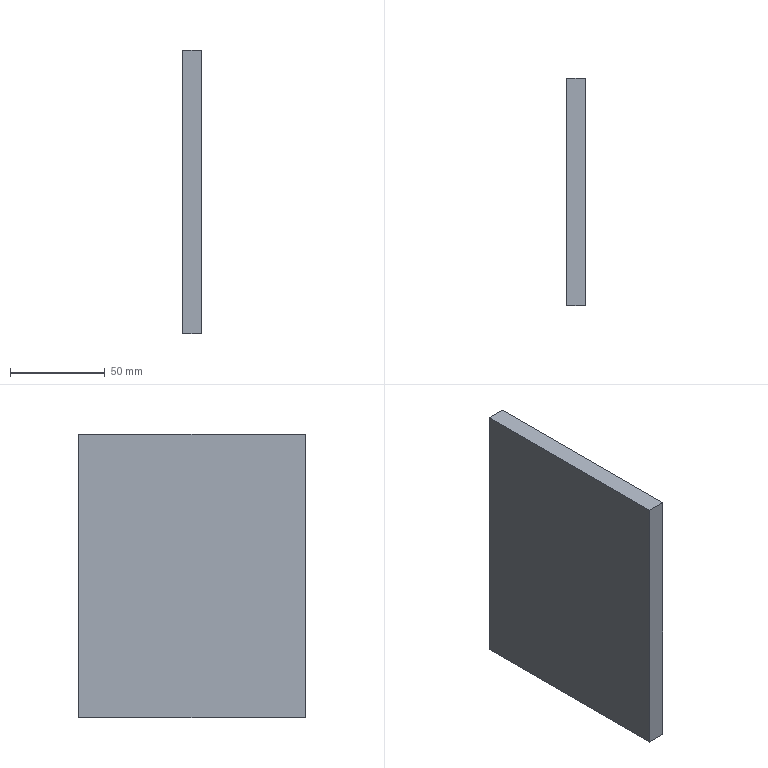Part | NX | 1 solid | 6 faces | box 10 x 120 x 150 mm | volume 180000 mm3 | plane 6
STEP:
#1=CARTESIAN_POINT('',(0.,-120.,0.));
#2=VERTEX_POINT('',#1);
#3=CARTESIAN_POINT('',(0.,-120.,-150.));
#4=VERTEX_POINT('',#3);
#5=CARTESIAN_POINT('',(0.,-120.,0.));
#6=DIRECTION('',(0.,0.,-1.));
#7=VECTOR('',#6,1.);
#8=LINE('',#5,#7);
#9=EDGE_CURVE('',#2,#4,#8,.T.);
#10=ORIENTED_EDGE('',*,*,#9,.T.);
#11=CARTESIAN_POINT('',(10.,-120.,-150.));
#12=VERTEX_POINT('',#11);
#13=CARTESIAN_POINT('',(10.,-120.,-150.));
#14=DIRECTION('',(-1.,0.,0.));
#15=VECTOR('',#14,1.);
#16=LINE('',#13,#15);
#17=EDGE_CURVE('',#12,#4,#16,.T.);
#18=ORIENTED_EDGE('',*,*,#17,.F.);
#19=CARTESIAN_POINT('',(10.,-120.,0.));
#20=VERTEX_POINT('',#19);
#21=CARTESIAN_POINT('',(10.,-120.,0.));
#22=DIRECTION('',(0.,0.,-1.));
#23=VECTOR('',#22,1.);
#24=LINE('',#21,#23);
#25=EDGE_CURVE('',#20,#12,#24,.T.);
#26=ORIENTED_EDGE('',*,*,#25,.F.);
#27=CARTESIAN_POINT('',(10.,-120.,0.));
#28=DIRECTION('',(-1.,0.,0.));
#29=VECTOR('',#28,1.);
#30=LINE('',#27,#29);
#31=EDGE_CURVE('',#20,#2,#30,.T.);
#32=ORIENTED_EDGE('',*,*,#31,.T.);
#33=EDGE_LOOP('',(#10,#18,#26,#32));
#34=FACE_OUTER_BOUND('',#33,.T.);
#35=CARTESIAN_POINT('',(10.,-120.,0.));
#36=DIRECTION('',(0.,1.,0.));
#37=DIRECTION('',(0.,0.,-1.));
#38=AXIS2_PLACEMENT_3D('',#35,#36,#37);
#39=PLANE('',#38);
#40=ADVANCED_FACE('',(#34),#39,.F.);
#41=CARTESIAN_POINT('',(0.,0.,-150.));
#42=VERTEX_POINT('',#41);
#43=CARTESIAN_POINT('',(0.,-120.,-150.));
#44=DIRECTION('',(0.,1.,0.));
#45=VECTOR('',#44,1.);
#46=LINE('',#43,#45);
#47=EDGE_CURVE('',#4,#42,#46,.T.);
#48=ORIENTED_EDGE('',*,*,#47,.T.);
#49=CARTESIAN_POINT('',(10.,0.,-150.));
#50=VERTEX_POINT('',#49);
#51=CARTESIAN_POINT('',(10.,0.,-150.));
#52=DIRECTION('',(-1.,0.,0.));
#53=VECTOR('',#52,1.);
#54=LINE('',#51,#53);
#55=EDGE_CURVE('',#50,#42,#54,.T.);
#56=ORIENTED_EDGE('',*,*,#55,.F.);
#57=CARTESIAN_POINT('',(10.,-120.,-150.));
#58=DIRECTION('',(0.,1.,0.));
#59=VECTOR('',#58,1.);
#60=LINE('',#57,#59);
#61=EDGE_CURVE('',#12,#50,#60,.T.);
#62=ORIENTED_EDGE('',*,*,#61,.F.);
#63=ORIENTED_EDGE('',*,*,#17,.T.);
#64=EDGE_LOOP('',(#48,#56,#62,#63));
#65=FACE_OUTER_BOUND('',#64,.T.);
#66=CARTESIAN_POINT('',(10.,-120.,-150.));
#67=DIRECTION('',(0.,0.,1.));
#68=DIRECTION('',(0.,1.,0.));
#69=AXIS2_PLACEMENT_3D('',#66,#67,#68);
#70=PLANE('',#69);
#71=ADVANCED_FACE('',(#65),#70,.F.);
#72=CARTESIAN_POINT('',(0.,0.,0.));
#73=VERTEX_POINT('',#72);
#74=CARTESIAN_POINT('',(0.,0.,-150.));
#75=DIRECTION('',(0.,0.,1.));
#76=VECTOR('',#75,1.);
#77=LINE('',#74,#76);
#78=EDGE_CURVE('',#42,#73,#77,.T.);
#79=ORIENTED_EDGE('',*,*,#78,.T.);
#80=CARTESIAN_POINT('',(10.,0.,0.));
#81=VERTEX_POINT('',#80);
#82=CARTESIAN_POINT('',(10.,0.,0.));
#83=DIRECTION('',(-1.,0.,0.));
#84=VECTOR('',#83,1.);
#85=LINE('',#82,#84);
#86=EDGE_CURVE('',#81,#73,#85,.T.);
#87=ORIENTED_EDGE('',*,*,#86,.F.);
#88=CARTESIAN_POINT('',(10.,0.,-150.));
#89=DIRECTION('',(0.,0.,1.));
#90=VECTOR('',#89,1.);
#91=LINE('',#88,#90);
#92=EDGE_CURVE('',#50,#81,#91,.T.);
#93=ORIENTED_EDGE('',*,*,#92,.F.);
#94=ORIENTED_EDGE('',*,*,#55,.T.);
#95=EDGE_LOOP('',(#79,#87,#93,#94));
#96=FACE_OUTER_BOUND('',#95,.T.);
#97=CARTESIAN_POINT('',(10.,0.,-150.));
#98=DIRECTION('',(0.,-1.,0.));
#99=DIRECTION('',(0.,0.,1.));
#100=AXIS2_PLACEMENT_3D('',#97,#98,#99);
#101=PLANE('',#100);
#102=ADVANCED_FACE('',(#96),#101,.F.);
#103=CARTESIAN_POINT('',(0.,0.,0.));
#104=DIRECTION('',(0.,-1.,0.));
#105=VECTOR('',#104,1.);
#106=LINE('',#103,#105);
#107=EDGE_CURVE('',#73,#2,#106,.T.);
#108=ORIENTED_EDGE('',*,*,#107,.T.);
#109=ORIENTED_EDGE('',*,*,#31,.F.);
#110=CARTESIAN_POINT('',(10.,0.,0.));
#111=DIRECTION('',(0.,-1.,0.));
#112=VECTOR('',#111,1.);
#113=LINE('',#110,#112);
#114=EDGE_CURVE('',#81,#20,#113,.T.);
#115=ORIENTED_EDGE('',*,*,#114,.F.);
#116=ORIENTED_EDGE('',*,*,#86,.T.);
#117=EDGE_LOOP('',(#108,#109,#115,#116));
#118=FACE_OUTER_BOUND('',#117,.T.);
#119=CARTESIAN_POINT('',(10.,0.,0.));
#120=DIRECTION('',(0.,0.,-1.));
#121=DIRECTION('',(0.,-1.,0.));
#122=AXIS2_PLACEMENT_3D('',#119,#120,#121);
#123=PLANE('',#122);
#124=ADVANCED_FACE('',(#118),#123,.F.);
#125=ORIENTED_EDGE('',*,*,#25,.T.);
#126=ORIENTED_EDGE('',*,*,#61,.T.);
#127=ORIENTED_EDGE('',*,*,#92,.T.);
#128=ORIENTED_EDGE('',*,*,#114,.T.);
#129=EDGE_LOOP('',(#125,#126,#127,#128));
#130=FACE_OUTER_BOUND('',#129,.T.);
#131=CARTESIAN_POINT('',(10.,0.,0.));
#132=DIRECTION('',(1.,0.,0.));
#133=DIRECTION('',(0.,0.,1.));
#134=AXIS2_PLACEMENT_3D('',#131,#132,#133);
#135=PLANE('',#134);
#136=ADVANCED_FACE('',(#130),#135,.T.);
#137=ORIENTED_EDGE('',*,*,#9,.F.);
#138=ORIENTED_EDGE('',*,*,#107,.F.);
#139=ORIENTED_EDGE('',*,*,#78,.F.);
#140=ORIENTED_EDGE('',*,*,#47,.F.);
#141=EDGE_LOOP('',(#137,#138,#139,#140));
#142=FACE_OUTER_BOUND('',#141,.T.);
#143=CARTESIAN_POINT('',(0.,0.,0.));
#144=DIRECTION('',(1.,0.,0.));
#145=DIRECTION('',(0.,0.,1.));
#146=AXIS2_PLACEMENT_3D('',#143,#144,#145);
#147=PLANE('',#146);
#148=ADVANCED_FACE('',(#142),#147,.F.);
#149=CLOSED_SHELL('',(#40,#71,#102,#124,#136,#148));
#150=MANIFOLD_SOLID_BREP('',#149);
#151=(LENGTH_UNIT()NAMED_UNIT(*)SI_UNIT(.MILLI.,.METRE.));
#152=UNCERTAINTY_MEASURE_WITH_UNIT(LENGTH_MEASURE(0.00002),#151,'','');
#153=(NAMED_UNIT(*)PLANE_ANGLE_UNIT()SI_UNIT($,.RADIAN.));
#154=PLANE_ANGLE_MEASURE_WITH_UNIT(PLANE_ANGLE_MEASURE(0.01745),#153);
#155=DIMENSIONAL_EXPONENTS(0.,0.,0.,0.,0.,0.,0.);
#156=(CONVERSION_BASED_UNIT('DEGREE',#154)NAMED_UNIT(#155)PLANE_ANGLE_UNIT());
#157=(NAMED_UNIT(*)SI_UNIT($,.STERADIAN.)SOLID_ANGLE_UNIT());
#158=(GEOMETRIC_REPRESENTATION_CONTEXT(3)GLOBAL_UNCERTAINTY_ASSIGNED_CONTEXT((#152))GLOBAL_UNIT_ASSIGNED_CONTEXT((#151,#156,#157))REPRESENTATION_CONTEXT('',''));
#159=ADVANCED_BREP_SHAPE_REPRESENTATION('',(#150),#158);